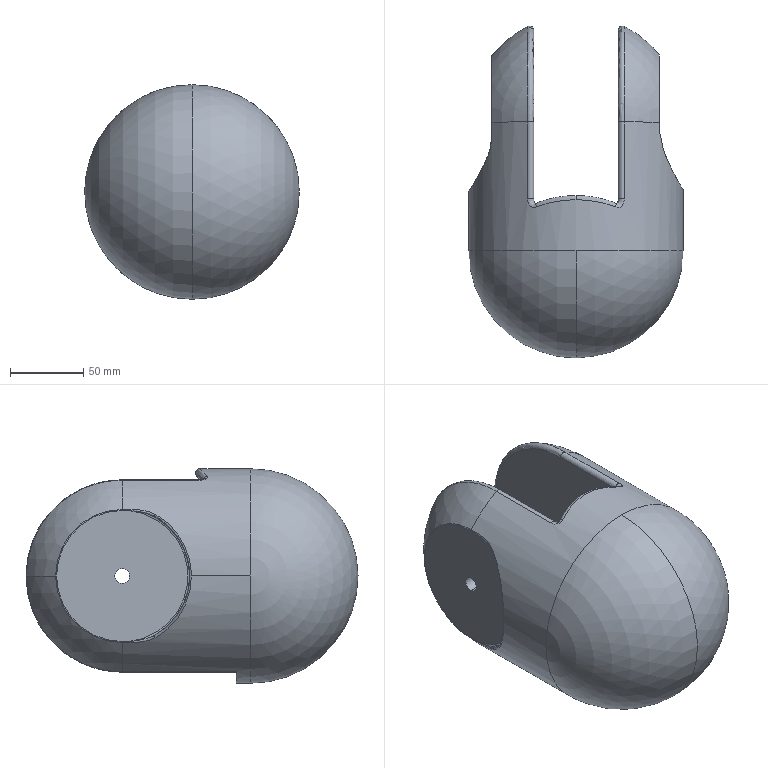Part | SolidWorks | features ICE 14, Fillet 4, Revolution 2, Scale 2 | 1 solid | 40 faces | box 146.538 x 226.907 x 146.538 mm | volume 1909002 mm3 | cylinder 16 | spline 7 | sphere 6 | plane 6 | torus 5 | commonest cylinder face diameters 5.769 x6 10.2 x4 2.308 x2 146.538 x2 92.308 x1 92.453 x1